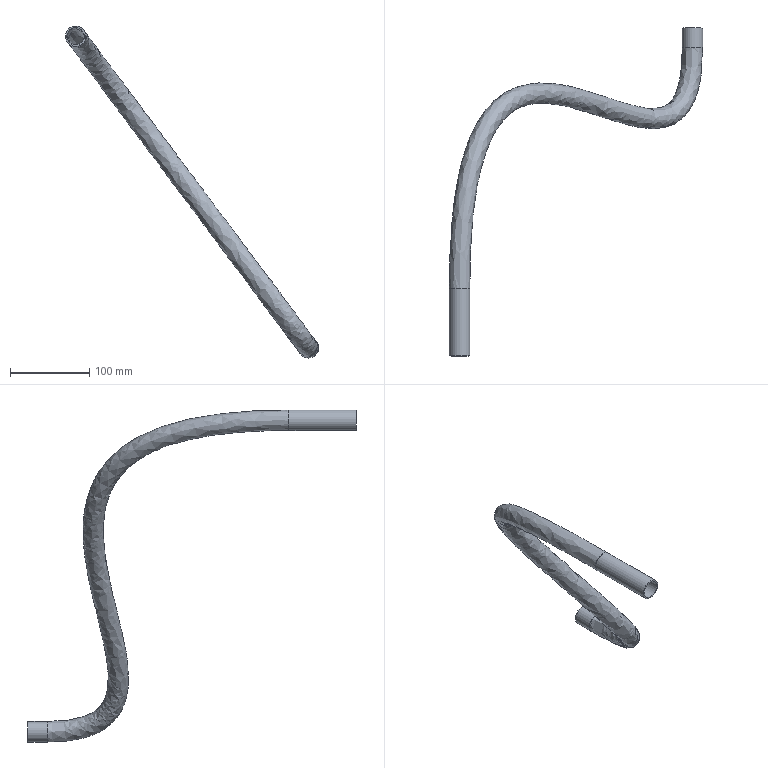Part | STEP file | Part 4^JBJ-F-0000-00 | 1 solid | 8 faces | box 320.031 x 414.992 x 419.382 mm | volume 125699 mm3 | cylinder 4 | spline 2 | plane 2 | commonest cylinder face diameters 22 x2 26 x2